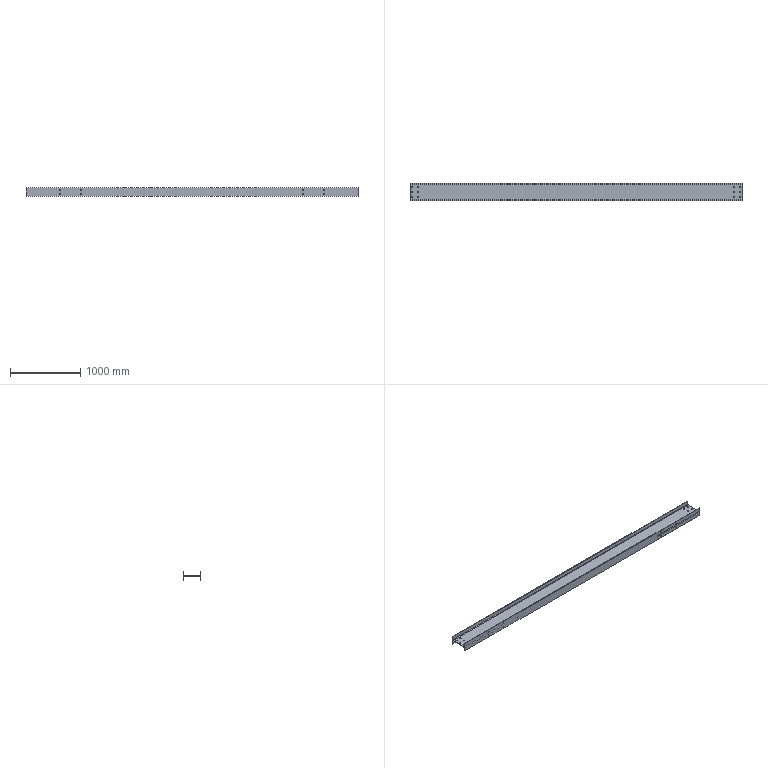Part | STEP file | 粉仓主梁2主体_Default<As Machined> | 1 solid | 58 faces | box 4730 x 250 x 125 mm | volume 17453380 mm3 | cylinder 44 | plane 14 | commonest cylinder face diameters 19 x24 15 x16 16 x4